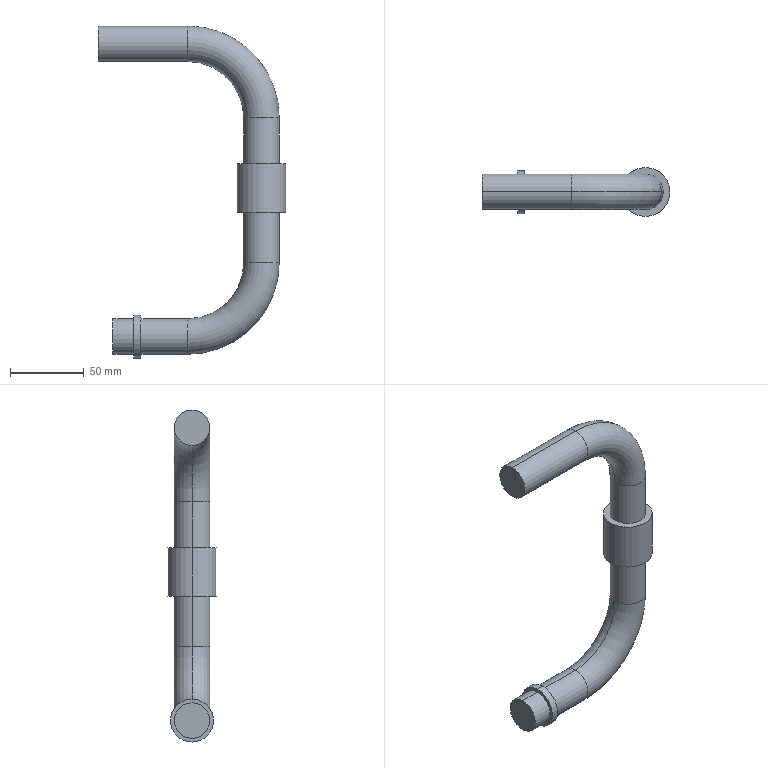Part | SolidWorks | features ICE 2, Sweep 1 | 1 solid | 24 faces | box 127 x 33 x 224.5 mm | volume 179947 mm3 | cylinder 14 | plane 6 | torus 4 | commonest cylinder face diameters 24 x10 29 x2 33 x2
STEP:
#1=CARTESIAN_POINT('',(60.5,0.,12.));
#2=VERTEX_POINT('',#1);
#3=CARTESIAN_POINT('',(60.5,0.,-12.));
#4=VERTEX_POINT('',#3);
#5=CARTESIAN_POINT('',(60.5,0.,0.));
#6=DIRECTION('',(-1.,0.,0.));
#7=DIRECTION('',(0.,0.,1.));
#8=AXIS2_PLACEMENT_3D('',#5,#6,#7);
#9=CIRCLE('',#8,12.);
#10=EDGE_CURVE('',#2,#4,#9,.T.);
#11=ORIENTED_EDGE('',*,*,#10,.F.);
#12=CARTESIAN_POINT('',(122.5,0.,-50.));
#13=VERTEX_POINT('',#12);
#14=CARTESIAN_POINT('',(60.5,0.,-50.));
#15=DIRECTION('',(0.,1.,0.));
#16=DIRECTION('',(0.,0.,1.));
#17=AXIS2_PLACEMENT_3D('',#14,#15,#16);
#18=CIRCLE('',#17,62.);
#19=EDGE_CURVE('',#2,#13,#18,.T.);
#20=ORIENTED_EDGE('',*,*,#19,.T.);
#21=CARTESIAN_POINT('',(98.5,0.,-50.));
#22=VERTEX_POINT('',#21);
#23=CARTESIAN_POINT('',(110.5,0.,-50.));
#24=DIRECTION('',(0.,0.,1.));
#25=DIRECTION('',(1.,0.,0.));
#26=AXIS2_PLACEMENT_3D('',#23,#24,#25);
#27=CIRCLE('',#26,12.);
#28=EDGE_CURVE('',#13,#22,#27,.T.);
#29=ORIENTED_EDGE('',*,*,#28,.T.);
#30=CARTESIAN_POINT('',(60.5,0.,-50.));
#31=DIRECTION('',(0.,1.,0.));
#32=DIRECTION('',(0.,0.,1.));
#33=AXIS2_PLACEMENT_3D('',#30,#31,#32);
#34=CIRCLE('',#33,38.);
#35=EDGE_CURVE('',#4,#22,#34,.T.);
#36=ORIENTED_EDGE('',*,*,#35,.F.);
#37=EDGE_LOOP('',(#11,#20,#29,#36));
#38=FACE_OUTER_BOUND('',#37,.T.);
#39=CARTESIAN_POINT('',(60.5,0.,-50.));
#40=DIRECTION('',(0.,1.,0.));
#41=DIRECTION('',(0.,0.,1.));
#42=AXIS2_PLACEMENT_3D('',#39,#40,#41);
#43=TOROIDAL_SURFACE('',#42,50.,12.);
#44=ADVANCED_FACE('',(#38),#43,.T.);
#45=CARTESIAN_POINT('',(122.5,0.,-148.));
#46=VERTEX_POINT('',#45);
#47=CARTESIAN_POINT('',(98.5,0.,-148.));
#48=VERTEX_POINT('',#47);
#49=CARTESIAN_POINT('',(110.5,0.,-148.));
#50=DIRECTION('',(0.,0.,1.));
#51=DIRECTION('',(1.,0.,0.));
#52=AXIS2_PLACEMENT_3D('',#49,#50,#51);
#53=CIRCLE('',#52,12.);
#54=EDGE_CURVE('',#46,#48,#53,.T.);
#55=ORIENTED_EDGE('',*,*,#54,.F.);
#56=CARTESIAN_POINT('',(60.5,0.,-210.));
#57=VERTEX_POINT('',#56);
#58=CARTESIAN_POINT('',(60.5,0.,-148.));
#59=DIRECTION('',(0.,1.,0.));
#60=DIRECTION('',(0.,0.,1.));
#61=AXIS2_PLACEMENT_3D('',#58,#59,#60);
#62=CIRCLE('',#61,62.);
#63=EDGE_CURVE('',#46,#57,#62,.T.);
#64=ORIENTED_EDGE('',*,*,#63,.T.);
#65=CARTESIAN_POINT('',(60.5,0.,-186.));
#66=VERTEX_POINT('',#65);
#67=CARTESIAN_POINT('',(60.5,0.,-198.));
#68=DIRECTION('',(1.,0.,0.));
#69=DIRECTION('',(0.,0.,-1.));
#70=AXIS2_PLACEMENT_3D('',#67,#68,#69);
#71=CIRCLE('',#70,12.);
#72=EDGE_CURVE('',#57,#66,#71,.T.);
#73=ORIENTED_EDGE('',*,*,#72,.T.);
#74=CARTESIAN_POINT('',(60.5,0.,-148.));
#75=DIRECTION('',(0.,1.,0.));
#76=DIRECTION('',(0.,0.,1.));
#77=AXIS2_PLACEMENT_3D('',#74,#75,#76);
#78=CIRCLE('',#77,38.);
#79=EDGE_CURVE('',#48,#66,#78,.T.);
#80=ORIENTED_EDGE('',*,*,#79,.F.);
#81=EDGE_LOOP('',(#55,#64,#73,#80));
#82=FACE_OUTER_BOUND('',#81,.T.);
#83=CARTESIAN_POINT('',(60.5,0.,-148.));
#84=DIRECTION('',(0.,1.,0.));
#85=DIRECTION('',(0.,0.,1.));
#86=AXIS2_PLACEMENT_3D('',#83,#84,#85);
#87=TOROIDAL_SURFACE('',#86,50.,12.);
#88=ADVANCED_FACE('',(#82),#87,.T.);
#89=ORIENTED_EDGE('',*,*,#28,.F.);
#90=CARTESIAN_POINT('',(122.5,0.,-81.));
#91=VERTEX_POINT('',#90);
#92=CARTESIAN_POINT('',(122.5,0.,-50.));
#93=DIRECTION('',(0.,0.,-1.));
#94=VECTOR('',#93,1000.);
#95=LINE('',#92,#94);
#96=EDGE_CURVE('',#13,#91,#95,.T.);
#97=ORIENTED_EDGE('',*,*,#96,.T.);
#98=CARTESIAN_POINT('',(98.5,0.,-81.));
#99=VERTEX_POINT('',#98);
#100=CARTESIAN_POINT('',(110.5,0.,-81.));
#101=DIRECTION('',(0.,0.,1.));
#102=DIRECTION('',(1.,0.,0.));
#103=AXIS2_PLACEMENT_3D('',#100,#101,#102);
#104=CIRCLE('',#103,12.);
#105=EDGE_CURVE('',#91,#99,#104,.T.);
#106=ORIENTED_EDGE('',*,*,#105,.T.);
#107=CARTESIAN_POINT('',(98.5,0.,-50.));
#108=DIRECTION('',(0.,0.,-1.));
#109=VECTOR('',#108,1000.);
#110=LINE('',#107,#109);
#111=EDGE_CURVE('',#22,#99,#110,.T.);
#112=ORIENTED_EDGE('',*,*,#111,.F.);
#113=EDGE_LOOP('',(#89,#97,#106,#112));
#114=FACE_OUTER_BOUND('',#113,.T.);
#115=CARTESIAN_POINT('',(110.5,0.,-50.));
#116=DIRECTION('',(0.,0.,-1.));
#117=DIRECTION('',(-1.,0.,0.));
#118=AXIS2_PLACEMENT_3D('',#115,#116,#117);
#119=CYLINDRICAL_SURFACE('',#118,12.);
#120=ADVANCED_FACE('',(#114),#119,.T.);
#121=CARTESIAN_POINT('',(0.,0.,12.));
#122=VERTEX_POINT('',#121);
#123=CARTESIAN_POINT('',(0.,0.,-12.));
#124=VERTEX_POINT('',#123);
#125=CARTESIAN_POINT('',(0.,0.,0.));
#126=DIRECTION('',(-1.,0.,0.));
#127=DIRECTION('',(0.,0.,1.));
#128=AXIS2_PLACEMENT_3D('',#125,#126,#127);
#129=CIRCLE('',#128,12.);
#130=EDGE_CURVE('',#122,#124,#129,.T.);
#131=ORIENTED_EDGE('',*,*,#130,.F.);
#132=CARTESIAN_POINT('',(0.,0.,12.));
#133=DIRECTION('',(1.,0.,0.));
#134=VECTOR('',#133,1000.);
#135=LINE('',#132,#134);
#136=EDGE_CURVE('',#122,#2,#135,.T.);
#137=ORIENTED_EDGE('',*,*,#136,.T.);
#138=ORIENTED_EDGE('',*,*,#10,.T.);
#139=CARTESIAN_POINT('',(0.,0.,-12.));
#140=DIRECTION('',(1.,0.,0.));
#141=VECTOR('',#140,1000.);
#142=LINE('',#139,#141);
#143=EDGE_CURVE('',#124,#4,#142,.T.);
#144=ORIENTED_EDGE('',*,*,#143,.F.);
#145=EDGE_LOOP('',(#131,#137,#138,#144));
#146=FACE_OUTER_BOUND('',#145,.T.);
#147=CARTESIAN_POINT('',(0.,0.,0.));
#148=DIRECTION('',(1.,0.,0.));
#149=DIRECTION('',(0.,0.,-1.));
#150=AXIS2_PLACEMENT_3D('',#147,#148,#149);
#151=CYLINDRICAL_SURFACE('',#150,12.);
#152=ADVANCED_FACE('',(#146),#151,.T.);
#153=CARTESIAN_POINT('',(127.,0.,-81.));
#154=VERTEX_POINT('',#153);
#155=CARTESIAN_POINT('',(94.,0.,-81.));
#156=VERTEX_POINT('',#155);
#157=CARTESIAN_POINT('',(110.5,0.,-81.));
#158=DIRECTION('',(0.,0.,1.));
#159=DIRECTION('',(1.,0.,0.));
#160=AXIS2_PLACEMENT_3D('',#157,#158,#159);
#161=CIRCLE('',#160,16.5);
#162=EDGE_CURVE('',#154,#156,#161,.T.);
#163=ORIENTED_EDGE('',*,*,#162,.F.);
#164=CARTESIAN_POINT('',(127.,0.,-114.));
#165=VERTEX_POINT('',#164);
#166=CARTESIAN_POINT('',(127.,0.,-81.));
#167=DIRECTION('',(0.,0.,-1.));
#168=VECTOR('',#167,1000.);
#169=LINE('',#166,#168);
#170=EDGE_CURVE('',#154,#165,#169,.T.);
#171=ORIENTED_EDGE('',*,*,#170,.T.);
#172=CARTESIAN_POINT('',(94.,0.,-114.));
#173=VERTEX_POINT('',#172);
#174=CARTESIAN_POINT('',(110.5,0.,-114.));
#175=DIRECTION('',(0.,0.,1.));
#176=DIRECTION('',(1.,0.,0.));
#177=AXIS2_PLACEMENT_3D('',#174,#175,#176);
#178=CIRCLE('',#177,16.5);
#179=EDGE_CURVE('',#165,#173,#178,.T.);
#180=ORIENTED_EDGE('',*,*,#179,.T.);
#181=CARTESIAN_POINT('',(94.,0.,-81.));
#182=DIRECTION('',(0.,0.,-1.));
#183=VECTOR('',#182,1000.);
#184=LINE('',#181,#183);
#185=EDGE_CURVE('',#156,#173,#184,.T.);
#186=ORIENTED_EDGE('',*,*,#185,.F.);
#187=EDGE_LOOP('',(#163,#171,#180,#186));
#188=FACE_OUTER_BOUND('',#187,.T.);
#189=CARTESIAN_POINT('',(110.5,0.,-81.));
#190=DIRECTION('',(0.,0.,-1.));
#191=DIRECTION('',(-1.,0.,0.));
#192=AXIS2_PLACEMENT_3D('',#189,#190,#191);
#193=CYLINDRICAL_SURFACE('',#192,16.5);
#194=ADVANCED_FACE('',(#188),#193,.T.);
#195=CARTESIAN_POINT('',(24.,0.,-186.));
#196=VERTEX_POINT('',#195);
#197=CARTESIAN_POINT('',(24.,0.,-210.));
#198=VERTEX_POINT('',#197);
#199=CARTESIAN_POINT('',(24.,0.,-198.));
#200=DIRECTION('',(-1.,0.,0.));
#201=DIRECTION('',(0.,0.,1.));
#202=AXIS2_PLACEMENT_3D('',#199,#200,#201);
#203=CIRCLE('',#202,12.);
#204=EDGE_CURVE('',#196,#198,#203,.T.);
#205=ORIENTED_EDGE('',*,*,#204,.T.);
#206=CARTESIAN_POINT('',(10.,0.,-210.));
#207=VERTEX_POINT('',#206);
#208=CARTESIAN_POINT('',(60.5,0.,-210.));
#209=DIRECTION('',(-1.,0.,0.));
#210=VECTOR('',#209,1000.);
#211=LINE('',#208,#210);
#212=EDGE_CURVE('',#198,#207,#211,.T.);
#213=ORIENTED_EDGE('',*,*,#212,.T.);
#214=CARTESIAN_POINT('',(10.,0.,-186.));
#215=VERTEX_POINT('',#214);
#216=CARTESIAN_POINT('',(10.,0.,-198.));
#217=DIRECTION('',(1.,0.,0.));
#218=DIRECTION('',(0.,0.,-1.));
#219=AXIS2_PLACEMENT_3D('',#216,#217,#218);
#220=CIRCLE('',#219,12.);
#221=EDGE_CURVE('',#207,#215,#220,.T.);
#222=ORIENTED_EDGE('',*,*,#221,.T.);
#223=CARTESIAN_POINT('',(60.5,0.,-186.));
#224=DIRECTION('',(-1.,0.,0.));
#225=VECTOR('',#224,1000.);
#226=LINE('',#223,#225);
#227=EDGE_CURVE('',#196,#215,#226,.T.);
#228=ORIENTED_EDGE('',*,*,#227,.F.);
#229=EDGE_LOOP('',(#205,#213,#222,#228));
#230=FACE_OUTER_BOUND('',#229,.T.);
#231=CARTESIAN_POINT('',(60.5,0.,-198.));
#232=DIRECTION('',(-1.,0.,0.));
#233=DIRECTION('',(0.,0.,1.));
#234=AXIS2_PLACEMENT_3D('',#231,#232,#233);
#235=CYLINDRICAL_SURFACE('',#234,12.);
#236=ADVANCED_FACE('',(#230),#235,.T.);
#237=CARTESIAN_POINT('',(29.,0.,-183.5));
#238=VERTEX_POINT('',#237);
#239=CARTESIAN_POINT('',(29.,0.,-212.5));
#240=VERTEX_POINT('',#239);
#241=CARTESIAN_POINT('',(29.,0.,-198.));
#242=DIRECTION('',(-1.,0.,0.));
#243=DIRECTION('',(0.,0.,1.));
#244=AXIS2_PLACEMENT_3D('',#241,#242,#243);
#245=CIRCLE('',#244,14.5);
#246=EDGE_CURVE('',#238,#240,#245,.T.);
#247=ORIENTED_EDGE('',*,*,#246,.T.);
#248=CARTESIAN_POINT('',(24.,0.,-212.5));
#249=VERTEX_POINT('',#248);
#250=CARTESIAN_POINT('',(29.,0.,-212.5));
#251=DIRECTION('',(-1.,0.,0.));
#252=VECTOR('',#251,1000.);
#253=LINE('',#250,#252);
#254=EDGE_CURVE('',#240,#249,#253,.T.);
#255=ORIENTED_EDGE('',*,*,#254,.T.);
#256=CARTESIAN_POINT('',(24.,0.,-183.5));
#257=VERTEX_POINT('',#256);
#258=CARTESIAN_POINT('',(24.,0.,-198.));
#259=DIRECTION('',(-1.,0.,0.));
#260=DIRECTION('',(0.,0.,1.));
#261=AXIS2_PLACEMENT_3D('',#258,#259,#260);
#262=CIRCLE('',#261,14.5);
#263=EDGE_CURVE('',#257,#249,#262,.T.);
#264=ORIENTED_EDGE('',*,*,#263,.F.);
#265=CARTESIAN_POINT('',(29.,0.,-183.5));
#266=DIRECTION('',(-1.,0.,0.));
#267=VECTOR('',#266,1000.);
#268=LINE('',#265,#267);
#269=EDGE_CURVE('',#238,#257,#268,.T.);
#270=ORIENTED_EDGE('',*,*,#269,.F.);
#271=EDGE_LOOP('',(#247,#255,#264,#270));
#272=FACE_OUTER_BOUND('',#271,.T.);
#273=CARTESIAN_POINT('',(29.,0.,-198.));
#274=DIRECTION('',(-1.,0.,0.));
#275=DIRECTION('',(0.,0.,1.));
#276=AXIS2_PLACEMENT_3D('',#273,#274,#275);
#277=CYLINDRICAL_SURFACE('',#276,14.5);
#278=ADVANCED_FACE('',(#272),#277,.T.);
#279=ORIENTED_EDGE('',*,*,#72,.F.);
#280=CARTESIAN_POINT('',(29.,0.,-210.));
#281=VERTEX_POINT('',#280);
#282=CARTESIAN_POINT('',(60.5,0.,-210.));
#283=DIRECTION('',(-1.,0.,0.));
#284=VECTOR('',#283,1000.);
#285=LINE('',#282,#284);
#286=EDGE_CURVE('',#57,#281,#285,.T.);
#287=ORIENTED_EDGE('',*,*,#286,.T.);
#288=CARTESIAN_POINT('',(29.,0.,-186.));
#289=VERTEX_POINT('',#288);
#290=CARTESIAN_POINT('',(29.,0.,-198.));
#291=DIRECTION('',(-1.,0.,0.));
#292=DIRECTION('',(0.,0.,1.));
#293=AXIS2_PLACEMENT_3D('',#290,#291,#292);
#294=CIRCLE('',#293,12.);
#295=EDGE_CURVE('',#289,#281,#294,.T.);
#296=ORIENTED_EDGE('',*,*,#295,.F.);
#297=CARTESIAN_POINT('',(60.5,0.,-186.));
#298=DIRECTION('',(-1.,0.,0.));
#299=VECTOR('',#298,1000.);
#300=LINE('',#297,#299);
#301=EDGE_CURVE('',#66,#289,#300,.T.);
#302=ORIENTED_EDGE('',*,*,#301,.F.);
#303=EDGE_LOOP('',(#279,#287,#296,#302));
#304=FACE_OUTER_BOUND('',#303,.T.);
#305=CARTESIAN_POINT('',(60.5,0.,-198.));
#306=DIRECTION('',(-1.,0.,0.));
#307=DIRECTION('',(0.,0.,1.));
#308=AXIS2_PLACEMENT_3D('',#305,#306,#307);
#309=CYLINDRICAL_SURFACE('',#308,12.);
#310=ADVANCED_FACE('',(#304),#309,.T.);
#311=CARTESIAN_POINT('',(122.5,0.,-114.));
#312=VERTEX_POINT('',#311);
#313=CARTESIAN_POINT('',(98.5,0.,-114.));
#314=VERTEX_POINT('',#313);
#315=CARTESIAN_POINT('',(110.5,0.,-114.));
#316=DIRECTION('',(0.,0.,1.));
#317=DIRECTION('',(1.,0.,0.));
#318=AXIS2_PLACEMENT_3D('',#315,#316,#317);
#319=CIRCLE('',#318,12.);
#320=EDGE_CURVE('',#312,#314,#319,.T.);
#321=ORIENTED_EDGE('',*,*,#320,.F.);
#322=CARTESIAN_POINT('',(122.5,0.,-50.));
#323=DIRECTION('',(0.,0.,-1.));
#324=VECTOR('',#323,1000.);
#325=LINE('',#322,#324);
#326=EDGE_CURVE('',#312,#46,#325,.T.);
#327=ORIENTED_EDGE('',*,*,#326,.T.);
#328=ORIENTED_EDGE('',*,*,#54,.T.);
#329=CARTESIAN_POINT('',(98.5,0.,-50.));
#330=DIRECTION('',(0.,0.,-1.));
#331=VECTOR('',#330,1000.);
#332=LINE('',#329,#331);
#333=EDGE_CURVE('',#314,#48,#332,.T.);
#334=ORIENTED_EDGE('',*,*,#333,.F.);
#335=EDGE_LOOP('',(#321,#327,#328,#334));
#336=FACE_OUTER_BOUND('',#335,.T.);
#337=CARTESIAN_POINT('',(110.5,0.,-50.));
#338=DIRECTION('',(0.,0.,-1.));
#339=DIRECTION('',(-1.,0.,0.));
#340=AXIS2_PLACEMENT_3D('',#337,#338,#339);
#341=CYLINDRICAL_SURFACE('',#340,12.);
#342=ADVANCED_FACE('',(#336),#341,.T.);
#343=ORIENTED_EDGE('',*,*,#326,.F.);
#344=CARTESIAN_POINT('',(110.5,0.,-114.));
#345=DIRECTION('',(0.,0.,1.));
#346=DIRECTION('',(1.,0.,0.));
#347=AXIS2_PLACEMENT_3D('',#344,#345,#346);
#348=CIRCLE('',#347,12.);
#349=EDGE_CURVE('',#314,#312,#348,.T.);
#350=ORIENTED_EDGE('',*,*,#349,.F.);
#351=ORIENTED_EDGE('',*,*,#333,.T.);
#352=CARTESIAN_POINT('',(110.5,0.,-148.));
#353=DIRECTION('',(0.,0.,1.));
#354=DIRECTION('',(1.,0.,0.));
#355=AXIS2_PLACEMENT_3D('',#352,#353,#354);
#356=CIRCLE('',#355,12.);
#357=EDGE_CURVE('',#48,#46,#356,.T.);
#358=ORIENTED_EDGE('',*,*,#357,.T.);
#359=EDGE_LOOP('',(#343,#350,#351,#358));
#360=FACE_OUTER_BOUND('',#359,.T.);
#361=CARTESIAN_POINT('',(110.5,0.,-50.));
#362=DIRECTION('',(0.,0.,-1.));
#363=DIRECTION('',(-1.,0.,0.));
#364=AXIS2_PLACEMENT_3D('',#361,#362,#363);
#365=CYLINDRICAL_SURFACE('',#364,12.);
#366=ADVANCED_FACE('',(#360),#365,.T.);
#367=ORIENTED_EDGE('',*,*,#286,.F.);
#368=CARTESIAN_POINT('',(60.5,0.,-198.));
#369=DIRECTION('',(1.,0.,0.));
#370=DIRECTION('',(0.,0.,-1.));
#371=AXIS2_PLACEMENT_3D('',#368,#369,#370);
#372=CIRCLE('',#371,12.);
#373=EDGE_CURVE('',#66,#57,#372,.T.);
#374=ORIENTED_EDGE('',*,*,#373,.F.);
#375=ORIENTED_EDGE('',*,*,#301,.T.);
#376=CARTESIAN_POINT('',(29.,0.,-198.));
#377=DIRECTION('',(-1.,0.,0.));
#378=DIRECTION('',(0.,0.,1.));
#379=AXIS2_PLACEMENT_3D('',#376,#377,#378);
#380=CIRCLE('',#379,12.);
#381=EDGE_CURVE('',#281,#289,#380,.T.);
#382=ORIENTED_EDGE('',*,*,#381,.F.);
#383=EDGE_LOOP('',(#367,#374,#375,#382));
#384=FACE_OUTER_BOUND('',#383,.T.);
#385=CARTESIAN_POINT('',(60.5,0.,-198.));
#386=DIRECTION('',(-1.,0.,0.));
#387=DIRECTION('',(0.,0.,1.));
#388=AXIS2_PLACEMENT_3D('',#385,#386,#387);
#389=CYLINDRICAL_SURFACE('',#388,12.);
#390=ADVANCED_FACE('',(#384),#389,.T.);
#391=ORIENTED_EDGE('',*,*,#63,.F.);
#392=ORIENTED_EDGE('',*,*,#357,.F.);
#393=ORIENTED_EDGE('',*,*,#79,.T.);
#394=ORIENTED_EDGE('',*,*,#373,.T.);
#395=EDGE_LOOP('',(#391,#392,#393,#394));
#396=FACE_OUTER_BOUND('',#395,.T.);
#397=CARTESIAN_POINT('',(60.5,0.,-148.));
#398=DIRECTION('',(0.,1.,0.));
#399=DIRECTION('',(0.,0.,1.));
#400=AXIS2_PLACEMENT_3D('',#397,#398,#399);
#401=TOROIDAL_SURFACE('',#400,50.,12.);
#402=ADVANCED_FACE('',(#396),#401,.T.);
#403=ORIENTED_EDGE('',*,*,#254,.F.);
#404=CARTESIAN_POINT('',(29.,0.,-198.));
#405=DIRECTION('',(-1.,0.,0.));
#406=DIRECTION('',(0.,0.,1.));
#407=AXIS2_PLACEMENT_3D('',#404,#405,#406);
#408=CIRCLE('',#407,14.5);
#409=EDGE_CURVE('',#240,#238,#408,.T.);
#410=ORIENTED_EDGE('',*,*,#409,.T.);
#411=ORIENTED_EDGE('',*,*,#269,.T.);
#412=CARTESIAN_POINT('',(24.,0.,-198.));
#413=DIRECTION('',(-1.,0.,0.));
#414=DIRECTION('',(0.,0.,1.));
#415=AXIS2_PLACEMENT_3D('',#412,#413,#414);
#416=CIRCLE('',#415,14.5);
#417=EDGE_CURVE('',#249,#257,#416,.T.);
#418=ORIENTED_EDGE('',*,*,#417,.F.);
#419=EDGE_LOOP('',(#403,#410,#411,#418));
#420=FACE_OUTER_BOUND('',#419,.T.);
#421=CARTESIAN_POINT('',(29.,0.,-198.));
#422=DIRECTION('',(-1.,0.,0.));
#423=DIRECTION('',(0.,0.,1.));
#424=AXIS2_PLACEMENT_3D('',#421,#422,#423);
#425=CYLINDRICAL_SURFACE('',#424,14.5);
#426=ADVANCED_FACE('',(#420),#425,.T.);
#427=ORIENTED_EDGE('',*,*,#295,.T.);
#428=ORIENTED_EDGE('',*,*,#381,.T.);
#429=EDGE_LOOP('',(#427,#428));
#430=FACE_BOUND('',#429,.T.);
#431=ORIENTED_EDGE('',*,*,#246,.F.);
#432=ORIENTED_EDGE('',*,*,#409,.F.);
#433=EDGE_LOOP('',(#431,#432));
#434=FACE_OUTER_BOUND('',#433,.T.);
#435=CARTESIAN_POINT('',(29.,0.,-198.));
#436=DIRECTION('',(-1.,0.,0.));
#437=DIRECTION('',(0.,0.,1.));
#438=AXIS2_PLACEMENT_3D('',#435,#436,#437);
#439=PLANE('',#438);
#440=ADVANCED_FACE('',(#430,#434),#439,.F.);
#441=ORIENTED_EDGE('',*,*,#204,.F.);
#442=CARTESIAN_POINT('',(24.,0.,-198.));
#443=DIRECTION('',(-1.,0.,0.));
#444=DIRECTION('',(0.,0.,1.));
#445=AXIS2_PLACEMENT_3D('',#442,#443,#444);
#446=CIRCLE('',#445,12.);
#447=EDGE_CURVE('',#198,#196,#446,.T.);
#448=ORIENTED_EDGE('',*,*,#447,.F.);
#449=EDGE_LOOP('',(#441,#448));
#450=FACE_BOUND('',#449,.T.);
#451=ORIENTED_EDGE('',*,*,#263,.T.);
#452=ORIENTED_EDGE('',*,*,#417,.T.);
#453=EDGE_LOOP('',(#451,#452));
#454=FACE_OUTER_BOUND('',#453,.T.);
#455=CARTESIAN_POINT('',(24.,0.,-198.));
#456=DIRECTION('',(-1.,0.,0.));
#457=DIRECTION('',(0.,0.,1.));
#458=AXIS2_PLACEMENT_3D('',#455,#456,#457);
#459=PLANE('',#458);
#460=ADVANCED_FACE('',(#450,#454),#459,.T.);
#461=CARTESIAN_POINT('',(10.,0.,-198.));
#462=DIRECTION('',(1.,0.,0.));
#463=DIRECTION('',(0.,0.,-1.));
#464=AXIS2_PLACEMENT_3D('',#461,#462,#463);
#465=CIRCLE('',#464,12.);
#466=EDGE_CURVE('',#215,#207,#465,.T.);
#467=ORIENTED_EDGE('',*,*,#466,.F.);
#468=ORIENTED_EDGE('',*,*,#221,.F.);
#469=EDGE_LOOP('',(#467,#468));
#470=FACE_OUTER_BOUND('',#469,.T.);
#471=CARTESIAN_POINT('',(10.,0.,-198.));
#472=DIRECTION('',(1.,0.,0.));
#473=DIRECTION('',(0.,0.,-1.));
#474=AXIS2_PLACEMENT_3D('',#471,#472,#473);
#475=PLANE('',#474);
#476=ADVANCED_FACE('',(#470),#475,.F.);
#477=ORIENTED_EDGE('',*,*,#212,.F.);
#478=ORIENTED_EDGE('',*,*,#447,.T.);
#479=ORIENTED_EDGE('',*,*,#227,.T.);
#480=ORIENTED_EDGE('',*,*,#466,.T.);
#481=EDGE_LOOP('',(#477,#478,#479,#480));
#482=FACE_OUTER_BOUND('',#481,.T.);
#483=CARTESIAN_POINT('',(60.5,0.,-198.));
#484=DIRECTION('',(-1.,0.,0.));
#485=DIRECTION('',(0.,0.,1.));
#486=AXIS2_PLACEMENT_3D('',#483,#484,#485);
#487=CYLINDRICAL_SURFACE('',#486,12.);
#488=ADVANCED_FACE('',(#482),#487,.T.);
#489=ORIENTED_EDGE('',*,*,#170,.F.);
#490=CARTESIAN_POINT('',(110.5,0.,-81.));
#491=DIRECTION('',(0.,0.,1.));
#492=DIRECTION('',(1.,0.,0.));
#493=AXIS2_PLACEMENT_3D('',#490,#491,#492);
#494=CIRCLE('',#493,16.5);
#495=EDGE_CURVE('',#156,#154,#494,.T.);
#496=ORIENTED_EDGE('',*,*,#495,.F.);
#497=ORIENTED_EDGE('',*,*,#185,.T.);
#498=CARTESIAN_POINT('',(110.5,0.,-114.));
#499=DIRECTION('',(0.,0.,1.));
#500=DIRECTION('',(1.,0.,0.));
#501=AXIS2_PLACEMENT_3D('',#498,#499,#500);
#502=CIRCLE('',#501,16.5);
#503=EDGE_CURVE('',#173,#165,#502,.T.);
#504=ORIENTED_EDGE('',*,*,#503,.T.);
#505=EDGE_LOOP('',(#489,#496,#497,#504));
#506=FACE_OUTER_BOUND('',#505,.T.);
#507=CARTESIAN_POINT('',(110.5,0.,-81.));
#508=DIRECTION('',(0.,0.,-1.));
#509=DIRECTION('',(-1.,0.,0.));
#510=AXIS2_PLACEMENT_3D('',#507,#508,#509);
#511=CYLINDRICAL_SURFACE('',#510,16.5);
#512=ADVANCED_FACE('',(#506),#511,.T.);
#513=CARTESIAN_POINT('',(110.5,0.,-81.));
#514=DIRECTION('',(0.,0.,1.));
#515=DIRECTION('',(1.,0.,0.));
#516=AXIS2_PLACEMENT_3D('',#513,#514,#515);
#517=CIRCLE('',#516,12.);
#518=EDGE_CURVE('',#99,#91,#517,.T.);
#519=ORIENTED_EDGE('',*,*,#518,.F.);
#520=ORIENTED_EDGE('',*,*,#105,.F.);
#521=EDGE_LOOP('',(#519,#520));
#522=FACE_BOUND('',#521,.T.);
#523=ORIENTED_EDGE('',*,*,#495,.T.);
#524=ORIENTED_EDGE('',*,*,#162,.T.);
#525=EDGE_LOOP('',(#523,#524));
#526=FACE_OUTER_BOUND('',#525,.T.);
#527=CARTESIAN_POINT('',(110.5,0.,-81.));
#528=DIRECTION('',(0.,0.,1.));
#529=DIRECTION('',(1.,0.,0.));
#530=AXIS2_PLACEMENT_3D('',#527,#528,#529);
#531=PLANE('',#530);
#532=ADVANCED_FACE('',(#522,#526),#531,.T.);
#533=ORIENTED_EDGE('',*,*,#349,.T.);
#534=ORIENTED_EDGE('',*,*,#320,.T.);
#535=EDGE_LOOP('',(#533,#534));
#536=FACE_BOUND('',#535,.T.);
#537=ORIENTED_EDGE('',*,*,#503,.F.);
#538=ORIENTED_EDGE('',*,*,#179,.F.);
#539=EDGE_LOOP('',(#537,#538));
#540=FACE_OUTER_BOUND('',#539,.T.);
#541=CARTESIAN_POINT('',(110.5,0.,-114.));
#542=DIRECTION('',(0.,0.,1.));
#543=DIRECTION('',(1.,0.,0.));
#544=AXIS2_PLACEMENT_3D('',#541,#542,#543);
#545=PLANE('',#544);
#546=ADVANCED_FACE('',(#536,#540),#545,.F.);
#547=CARTESIAN_POINT('',(0.,0.,0.));
#548=DIRECTION('',(-1.,0.,0.));
#549=DIRECTION('',(0.,0.,1.));
#550=AXIS2_PLACEMENT_3D('',#547,#548,#549);
#551=CIRCLE('',#550,12.);
#552=EDGE_CURVE('',#124,#122,#551,.T.);
#553=ORIENTED_EDGE('',*,*,#552,.T.);
#554=ORIENTED_EDGE('',*,*,#130,.T.);
#555=EDGE_LOOP('',(#553,#554));
#556=FACE_OUTER_BOUND('',#555,.T.);
#557=CARTESIAN_POINT('',(0.,0.,0.));
#558=DIRECTION('',(-1.,0.,0.));
#559=DIRECTION('',(0.,0.,1.));
#560=AXIS2_PLACEMENT_3D('',#557,#558,#559);
#561=PLANE('',#560);
#562=ADVANCED_FACE('',(#556),#561,.T.);
#563=ORIENTED_EDGE('',*,*,#136,.F.);
#564=ORIENTED_EDGE('',*,*,#552,.F.);
#565=ORIENTED_EDGE('',*,*,#143,.T.);
#566=CARTESIAN_POINT('',(60.5,0.,0.));
#567=DIRECTION('',(-1.,0.,0.));
#568=DIRECTION('',(0.,0.,1.));
#569=AXIS2_PLACEMENT_3D('',#566,#567,#568);
#570=CIRCLE('',#569,12.);
#571=EDGE_CURVE('',#4,#2,#570,.T.);
#572=ORIENTED_EDGE('',*,*,#571,.T.);
#573=EDGE_LOOP('',(#563,#564,#565,#572));
#574=FACE_OUTER_BOUND('',#573,.T.);
#575=CARTESIAN_POINT('',(0.,0.,0.));
#576=DIRECTION('',(1.,0.,0.));
#577=DIRECTION('',(0.,0.,-1.));
#578=AXIS2_PLACEMENT_3D('',#575,#576,#577);
#579=CYLINDRICAL_SURFACE('',#578,12.);
#580=ADVANCED_FACE('',(#574),#579,.T.);
#581=ORIENTED_EDGE('',*,*,#19,.F.);
#582=ORIENTED_EDGE('',*,*,#571,.F.);
#583=ORIENTED_EDGE('',*,*,#35,.T.);
#584=CARTESIAN_POINT('',(110.5,0.,-50.));
#585=DIRECTION('',(0.,0.,1.));
#586=DIRECTION('',(1.,0.,0.));
#587=AXIS2_PLACEMENT_3D('',#584,#585,#586);
#588=CIRCLE('',#587,12.);
#589=EDGE_CURVE('',#22,#13,#588,.T.);
#590=ORIENTED_EDGE('',*,*,#589,.T.);
#591=EDGE_LOOP('',(#581,#582,#583,#590));
#592=FACE_OUTER_BOUND('',#591,.T.);
#593=CARTESIAN_POINT('',(60.5,0.,-50.));
#594=DIRECTION('',(0.,1.,0.));
#595=DIRECTION('',(0.,0.,1.));
#596=AXIS2_PLACEMENT_3D('',#593,#594,#595);
#597=TOROIDAL_SURFACE('',#596,50.,12.);
#598=ADVANCED_FACE('',(#592),#597,.T.);
#599=ORIENTED_EDGE('',*,*,#96,.F.);
#600=ORIENTED_EDGE('',*,*,#589,.F.);
#601=ORIENTED_EDGE('',*,*,#111,.T.);
#602=ORIENTED_EDGE('',*,*,#518,.T.);
#603=EDGE_LOOP('',(#599,#600,#601,#602));
#604=FACE_OUTER_BOUND('',#603,.T.);
#605=CARTESIAN_POINT('',(110.5,0.,-50.));
#606=DIRECTION('',(0.,0.,-1.));
#607=DIRECTION('',(-1.,0.,0.));
#608=AXIS2_PLACEMENT_3D('',#605,#606,#607);
#609=CYLINDRICAL_SURFACE('',#608,12.);
#610=ADVANCED_FACE('',(#604),#609,.T.);
#611=CLOSED_SHELL('',(#44,#88,#120,#152,#194,#236,#278,#310,#342,#366,#390,#402,#426,#440,#460,#476,#488,#512,#532,#546,#562,#580,#598,#610));
#612=MANIFOLD_SOLID_BREP('',#611);
#613=CARTESIAN_POINT('',(0.,0.,0.));
#614=DIRECTION('',(0.,0.,1.));
#615=DIRECTION('',(1.,0.,0.));
#616=AXIS2_PLACEMENT_3D('',#613,#614,#615);
#617=(LENGTH_UNIT()NAMED_UNIT(*)SI_UNIT(.MILLI.,.METRE.));
#618=UNCERTAINTY_MEASURE_WITH_UNIT(LENGTH_MEASURE(0.00001),#617,'','');
#619=(NAMED_UNIT(*)PLANE_ANGLE_UNIT()SI_UNIT($,.RADIAN.));
#620=(NAMED_UNIT(*)SI_UNIT($,.STERADIAN.)SOLID_ANGLE_UNIT());
#621=(GEOMETRIC_REPRESENTATION_CONTEXT(3)GLOBAL_UNCERTAINTY_ASSIGNED_CONTEXT((#618))GLOBAL_UNIT_ASSIGNED_CONTEXT((#617,#619,#620))REPRESENTATION_CONTEXT('',''));
#622=ADVANCED_BREP_SHAPE_REPRESENTATION('',(#612,#616),#621);